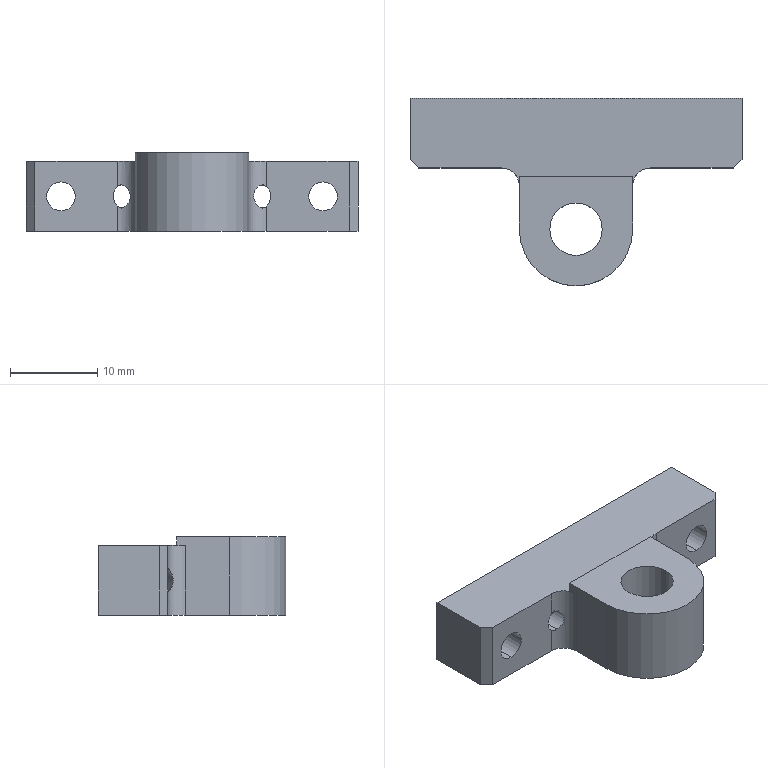Part | STEP file | PN_0022 | 1 solid | 32 faces | box 38 x 21.5 x 9 mm | volume 3334 mm3 | cylinder 13 | plane 13 | cone 6 | commonest cylinder face diameters 3 x4 3.3 x4 4 x2 6 x2 13 x1